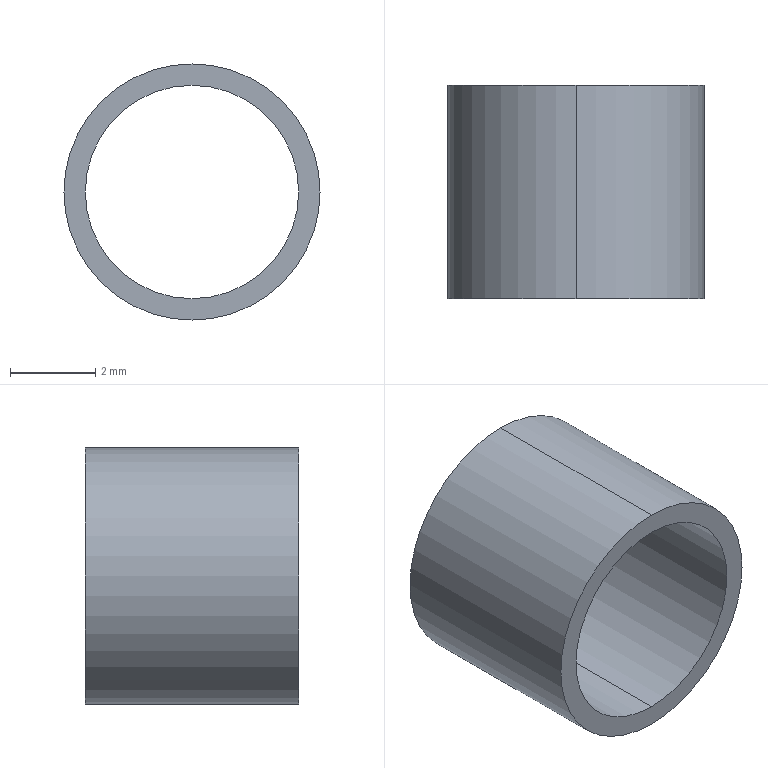Part | SolidWorks | features Extrusion 1 | 1 solid | 6 faces | box 6 x 5 x 6 mm | volume 43.197 mm3 | cylinder 4 | plane 2 | commonest cylinder face diameters 5 x2 6 x2
STEP:
#1=CARTESIAN_POINT('',(0.,5.,-2.5));
#2=VERTEX_POINT('',#1);
#3=CARTESIAN_POINT('',(0.,5.,2.5));
#4=VERTEX_POINT('',#3);
#5=CARTESIAN_POINT('',(0.,5.,0.));
#6=DIRECTION('',(0.,1.,0.));
#7=DIRECTION('',(0.,0.,1.));
#8=AXIS2_PLACEMENT_3D('',#5,#6,#7);
#9=CIRCLE('',#8,2.5);
#10=EDGE_CURVE('',#2,#4,#9,.T.);
#11=ORIENTED_EDGE('',*,*,#10,.T.);
#12=CARTESIAN_POINT('',(0.,0.,2.5));
#13=VERTEX_POINT('',#12);
#14=CARTESIAN_POINT('',(0.,5.,2.5));
#15=DIRECTION('',(0.,-1.,0.));
#16=VECTOR('',#15,1000.);
#17=LINE('',#14,#16);
#18=EDGE_CURVE('',#4,#13,#17,.T.);
#19=ORIENTED_EDGE('',*,*,#18,.T.);
#20=CARTESIAN_POINT('',(0.,0.,-2.5));
#21=VERTEX_POINT('',#20);
#22=CARTESIAN_POINT('',(0.,0.,0.));
#23=DIRECTION('',(0.,1.,0.));
#24=DIRECTION('',(0.,0.,1.));
#25=AXIS2_PLACEMENT_3D('',#22,#23,#24);
#26=CIRCLE('',#25,2.5);
#27=EDGE_CURVE('',#21,#13,#26,.T.);
#28=ORIENTED_EDGE('',*,*,#27,.F.);
#29=CARTESIAN_POINT('',(0.,5.,-2.5));
#30=DIRECTION('',(0.,-1.,0.));
#31=VECTOR('',#30,1000.);
#32=LINE('',#29,#31);
#33=EDGE_CURVE('',#2,#21,#32,.T.);
#34=ORIENTED_EDGE('',*,*,#33,.F.);
#35=EDGE_LOOP('',(#11,#19,#28,#34));
#36=FACE_OUTER_BOUND('',#35,.T.);
#37=CARTESIAN_POINT('',(0.,5.,0.));
#38=DIRECTION('',(0.,-1.,0.));
#39=DIRECTION('',(0.,0.,-1.));
#40=AXIS2_PLACEMENT_3D('',#37,#38,#39);
#41=CYLINDRICAL_SURFACE('',#40,2.5);
#42=ADVANCED_FACE('',(#36),#41,.F.);
#43=CARTESIAN_POINT('',(0.,5.,3.));
#44=VERTEX_POINT('',#43);
#45=CARTESIAN_POINT('',(0.,5.,-3.));
#46=VERTEX_POINT('',#45);
#47=CARTESIAN_POINT('',(0.,5.,0.));
#48=DIRECTION('',(0.,1.,0.));
#49=DIRECTION('',(0.,0.,1.));
#50=AXIS2_PLACEMENT_3D('',#47,#48,#49);
#51=CIRCLE('',#50,3.);
#52=EDGE_CURVE('',#44,#46,#51,.T.);
#53=ORIENTED_EDGE('',*,*,#52,.F.);
#54=CARTESIAN_POINT('',(0.,0.,3.));
#55=VERTEX_POINT('',#54);
#56=CARTESIAN_POINT('',(0.,5.,3.));
#57=DIRECTION('',(0.,-1.,0.));
#58=VECTOR('',#57,1000.);
#59=LINE('',#56,#58);
#60=EDGE_CURVE('',#44,#55,#59,.T.);
#61=ORIENTED_EDGE('',*,*,#60,.T.);
#62=CARTESIAN_POINT('',(0.,0.,-3.));
#63=VERTEX_POINT('',#62);
#64=CARTESIAN_POINT('',(0.,0.,0.));
#65=DIRECTION('',(0.,1.,0.));
#66=DIRECTION('',(0.,0.,1.));
#67=AXIS2_PLACEMENT_3D('',#64,#65,#66);
#68=CIRCLE('',#67,3.);
#69=EDGE_CURVE('',#55,#63,#68,.T.);
#70=ORIENTED_EDGE('',*,*,#69,.T.);
#71=CARTESIAN_POINT('',(0.,5.,-3.));
#72=DIRECTION('',(0.,-1.,0.));
#73=VECTOR('',#72,1000.);
#74=LINE('',#71,#73);
#75=EDGE_CURVE('',#46,#63,#74,.T.);
#76=ORIENTED_EDGE('',*,*,#75,.F.);
#77=EDGE_LOOP('',(#53,#61,#70,#76));
#78=FACE_OUTER_BOUND('',#77,.T.);
#79=CARTESIAN_POINT('',(0.,5.,0.));
#80=DIRECTION('',(0.,-1.,0.));
#81=DIRECTION('',(0.,0.,-1.));
#82=AXIS2_PLACEMENT_3D('',#79,#80,#81);
#83=CYLINDRICAL_SURFACE('',#82,3.);
#84=ADVANCED_FACE('',(#78),#83,.T.);
#85=CARTESIAN_POINT('',(0.,5.,0.));
#86=DIRECTION('',(0.,1.,0.));
#87=DIRECTION('',(0.,0.,1.));
#88=AXIS2_PLACEMENT_3D('',#85,#86,#87);
#89=CIRCLE('',#88,3.);
#90=EDGE_CURVE('',#46,#44,#89,.T.);
#91=ORIENTED_EDGE('',*,*,#90,.T.);
#92=ORIENTED_EDGE('',*,*,#52,.T.);
#93=EDGE_LOOP('',(#91,#92));
#94=FACE_OUTER_BOUND('',#93,.T.);
#95=ORIENTED_EDGE('',*,*,#10,.F.);
#96=CARTESIAN_POINT('',(0.,5.,0.));
#97=DIRECTION('',(0.,1.,0.));
#98=DIRECTION('',(0.,0.,1.));
#99=AXIS2_PLACEMENT_3D('',#96,#97,#98);
#100=CIRCLE('',#99,2.5);
#101=EDGE_CURVE('',#4,#2,#100,.T.);
#102=ORIENTED_EDGE('',*,*,#101,.F.);
#103=EDGE_LOOP('',(#95,#102));
#104=FACE_BOUND('',#103,.T.);
#105=CARTESIAN_POINT('',(0.,5.,0.));
#106=DIRECTION('',(0.,1.,0.));
#107=DIRECTION('',(0.,0.,1.));
#108=AXIS2_PLACEMENT_3D('',#105,#106,#107);
#109=PLANE('',#108);
#110=ADVANCED_FACE('',(#94,#104),#109,.T.);
#111=CARTESIAN_POINT('',(0.,0.,0.));
#112=DIRECTION('',(0.,1.,0.));
#113=DIRECTION('',(0.,0.,1.));
#114=AXIS2_PLACEMENT_3D('',#111,#112,#113);
#115=CIRCLE('',#114,3.);
#116=EDGE_CURVE('',#63,#55,#115,.T.);
#117=ORIENTED_EDGE('',*,*,#116,.F.);
#118=ORIENTED_EDGE('',*,*,#69,.F.);
#119=EDGE_LOOP('',(#117,#118));
#120=FACE_OUTER_BOUND('',#119,.T.);
#121=ORIENTED_EDGE('',*,*,#27,.T.);
#122=CARTESIAN_POINT('',(0.,0.,0.));
#123=DIRECTION('',(0.,1.,0.));
#124=DIRECTION('',(0.,0.,1.));
#125=AXIS2_PLACEMENT_3D('',#122,#123,#124);
#126=CIRCLE('',#125,2.5);
#127=EDGE_CURVE('',#13,#21,#126,.T.);
#128=ORIENTED_EDGE('',*,*,#127,.T.);
#129=EDGE_LOOP('',(#121,#128));
#130=FACE_BOUND('',#129,.T.);
#131=CARTESIAN_POINT('',(0.,0.,0.));
#132=DIRECTION('',(0.,1.,0.));
#133=DIRECTION('',(0.,0.,1.));
#134=AXIS2_PLACEMENT_3D('',#131,#132,#133);
#135=PLANE('',#134);
#136=ADVANCED_FACE('',(#120,#130),#135,.F.);
#137=ORIENTED_EDGE('',*,*,#60,.F.);
#138=ORIENTED_EDGE('',*,*,#90,.F.);
#139=ORIENTED_EDGE('',*,*,#75,.T.);
#140=ORIENTED_EDGE('',*,*,#116,.T.);
#141=EDGE_LOOP('',(#137,#138,#139,#140));
#142=FACE_OUTER_BOUND('',#141,.T.);
#143=CARTESIAN_POINT('',(0.,5.,0.));
#144=DIRECTION('',(0.,-1.,0.));
#145=DIRECTION('',(0.,0.,-1.));
#146=AXIS2_PLACEMENT_3D('',#143,#144,#145);
#147=CYLINDRICAL_SURFACE('',#146,3.);
#148=ADVANCED_FACE('',(#142),#147,.T.);
#149=ORIENTED_EDGE('',*,*,#18,.F.);
#150=ORIENTED_EDGE('',*,*,#101,.T.);
#151=ORIENTED_EDGE('',*,*,#33,.T.);
#152=ORIENTED_EDGE('',*,*,#127,.F.);
#153=EDGE_LOOP('',(#149,#150,#151,#152));
#154=FACE_OUTER_BOUND('',#153,.T.);
#155=CARTESIAN_POINT('',(0.,5.,0.));
#156=DIRECTION('',(0.,-1.,0.));
#157=DIRECTION('',(0.,0.,-1.));
#158=AXIS2_PLACEMENT_3D('',#155,#156,#157);
#159=CYLINDRICAL_SURFACE('',#158,2.5);
#160=ADVANCED_FACE('',(#154),#159,.F.);
#161=CLOSED_SHELL('',(#42,#84,#110,#136,#148,#160));
#162=MANIFOLD_SOLID_BREP('',#161);
#163=CARTESIAN_POINT('',(0.,0.,0.));
#164=DIRECTION('',(0.,0.,1.));
#165=DIRECTION('',(1.,0.,0.));
#166=AXIS2_PLACEMENT_3D('',#163,#164,#165);
#167=(LENGTH_UNIT()NAMED_UNIT(*)SI_UNIT(.MILLI.,.METRE.));
#168=UNCERTAINTY_MEASURE_WITH_UNIT(LENGTH_MEASURE(0.00001),#167,'','');
#169=(NAMED_UNIT(*)PLANE_ANGLE_UNIT()SI_UNIT($,.RADIAN.));
#170=(NAMED_UNIT(*)SI_UNIT($,.STERADIAN.)SOLID_ANGLE_UNIT());
#171=(GEOMETRIC_REPRESENTATION_CONTEXT(3)GLOBAL_UNCERTAINTY_ASSIGNED_CONTEXT((#168))GLOBAL_UNIT_ASSIGNED_CONTEXT((#167,#169,#170))REPRESENTATION_CONTEXT('',''));
#172=ADVANCED_BREP_SHAPE_REPRESENTATION('',(#162,#166),#171);